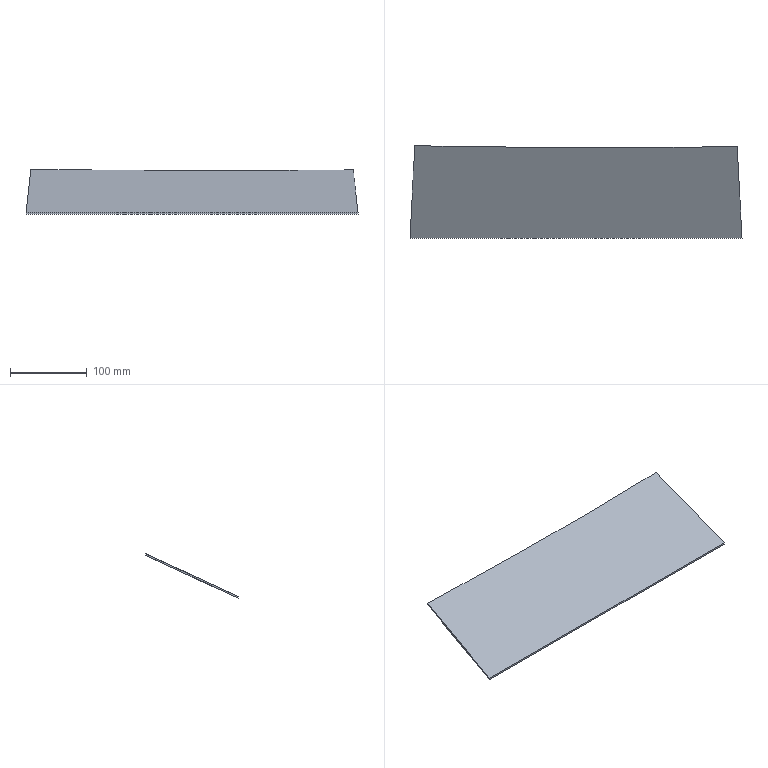Part | NX | features solid 2 | 1 solid | 6 faces | box 431.972 x 120.175 x 58.245 mm | volume 111226 mm3 | plane 5 | spline 1
STEP:
#1=CARTESIAN_POINT('',(-249.743,-364.825,19.75));
#2=VERTEX_POINT('',#1);
#3=CARTESIAN_POINT('',(169.68,-365.715,19.335));
#4=VERTEX_POINT('',#3);
#5=CARTESIAN_POINT('',(-249.743,-364.825,19.75));
#6=CARTESIAN_POINT('',(-232.267,-365.051,19.645));
#7=CARTESIAN_POINT('',(-206.054,-365.258,19.548));
#8=CARTESIAN_POINT('',(-171.103,-365.659,19.361));
#9=CARTESIAN_POINT('',(-136.154,-366.255,19.083));
#10=CARTESIAN_POINT('',(-101.203,-366.757,18.849));
#11=CARTESIAN_POINT('',(-66.253,-367.313,18.59));
#12=CARTESIAN_POINT('',(-40.041,-367.708,18.406));
#13=CARTESIAN_POINT('',(-13.826,-367.635,18.44));
#14=CARTESIAN_POINT('',(12.388,-367.617,18.448));
#15=CARTESIAN_POINT('',(38.602,-367.689,18.414));
#16=CARTESIAN_POINT('',(64.817,-367.364,18.566));
#17=CARTESIAN_POINT('',(91.033,-366.909,18.778));
#18=CARTESIAN_POINT('',(117.249,-366.489,18.974));
#19=CARTESIAN_POINT('',(143.464,-366.132,19.141));
#20=CARTESIAN_POINT('',(160.941,-365.843,19.275));
#21=CARTESIAN_POINT('',(169.68,-365.715,19.335));
#22=B_SPLINE_CURVE_WITH_KNOTS('',3,(#5,#6,#7,#8,#9,#10,#11,#12,#13,#14,#15,#16,#17,#18,#19,#20,#21),.UNSPECIFIED.,.F.,.F.,(4,1,1,1,1,1,1,1,1,1,1,1,1,1,4),(0.5223,0.5724,0.5974,0.6224,0.6725,0.6975,0.7226,0.7476,0.7726,0.7977,0.8227,0.8477,0.8727,0.8978,0.9228),.UNSPECIFIED.);
#23=EDGE_CURVE('',#2,#4,#22,.T.);
#24=ORIENTED_EDGE('',*,*,#23,.T.);
#25=CARTESIAN_POINT('',(169.68,-365.715,17.128));
#26=VERTEX_POINT('',#25);
#27=CARTESIAN_POINT('',(169.68,-365.715,18.403));
#28=DIRECTION('',(0.,0.,-1.));
#29=VECTOR('',#28,1000.);
#30=LINE('',#27,#29);
#31=EDGE_CURVE('',#4,#26,#30,.T.);
#32=ORIENTED_EDGE('',*,*,#31,.T.);
#33=CARTESIAN_POINT('',(-249.743,-364.825,17.543));
#34=VERTEX_POINT('',#33);
#35=CARTESIAN_POINT('',(-249.743,-364.825,17.543));
#36=CARTESIAN_POINT('',(-232.263,-365.051,17.438));
#37=CARTESIAN_POINT('',(-206.047,-365.258,17.342));
#38=CARTESIAN_POINT('',(-171.09,-365.659,17.154));
#39=CARTESIAN_POINT('',(-136.129,-366.256,16.876));
#40=CARTESIAN_POINT('',(-101.17,-366.757,16.642));
#41=CARTESIAN_POINT('',(-66.209,-367.314,16.383));
#42=CARTESIAN_POINT('',(-39.99,-367.709,16.199));
#43=CARTESIAN_POINT('',(-13.778,-367.634,16.233));
#44=CARTESIAN_POINT('',(12.435,-367.617,16.241));
#45=CARTESIAN_POINT('',(38.649,-367.689,16.208));
#46=CARTESIAN_POINT('',(64.856,-367.364,16.36));
#47=CARTESIAN_POINT('',(91.061,-366.909,16.572));
#48=CARTESIAN_POINT('',(117.267,-366.489,16.767));
#49=CARTESIAN_POINT('',(143.474,-366.131,16.934));
#50=CARTESIAN_POINT('',(160.944,-365.843,17.069));
#51=CARTESIAN_POINT('',(169.68,-365.715,17.128));
#52=B_SPLINE_CURVE_WITH_KNOTS('',3,(#35,#36,#37,#38,#39,#40,#41,#42,#43,#44,#45,#46,#47,#48,#49,#50,#51),.UNSPECIFIED.,.F.,.F.,(4,1,1,1,1,1,1,1,1,1,1,1,1,1,4),(0.5017,0.5492,0.573,0.5967,0.6442,0.6679,0.6917,0.7154,0.7392,0.7629,0.7867,0.8104,0.8342,0.8579,0.8816),.UNSPECIFIED.);
#53=EDGE_CURVE('',#34,#26,#52,.T.);
#54=ORIENTED_EDGE('',*,*,#53,.F.);
#55=CARTESIAN_POINT('',(-249.743,-364.825,32.28));
#56=DIRECTION('',(0.,0.,-1.));
#57=VECTOR('',#56,1000.);
#58=LINE('',#55,#57);
#59=EDGE_CURVE('',#34,#2,#58,.F.);
#60=ORIENTED_EDGE('',*,*,#59,.T.);
#61=EDGE_LOOP('',(#24,#32,#54,#60));
#62=FACE_BOUND('',#61,.T.);
#63=CARTESIAN_POINT('',(169.68,-365.715,19.773));
#64=CARTESIAN_POINT('',(169.68,-365.715,15.99));
#65=CARTESIAN_POINT('',(160.942,-365.843,19.773));
#66=CARTESIAN_POINT('',(160.942,-365.843,15.99));
#67=CARTESIAN_POINT('',(143.467,-366.132,19.773));
#68=CARTESIAN_POINT('',(143.467,-366.132,15.99));
#69=CARTESIAN_POINT('',(117.253,-366.489,19.773));
#70=CARTESIAN_POINT('',(117.253,-366.489,15.99));
#71=CARTESIAN_POINT('',(91.041,-366.909,19.773));
#72=CARTESIAN_POINT('',(91.041,-366.909,15.99));
#73=CARTESIAN_POINT('',(64.829,-367.364,19.773));
#74=CARTESIAN_POINT('',(64.829,-367.364,15.99));
#75=CARTESIAN_POINT('',(38.614,-367.689,19.773));
#76=CARTESIAN_POINT('',(38.614,-367.689,15.99));
#77=CARTESIAN_POINT('',(12.398,-367.617,19.773));
#78=CARTESIAN_POINT('',(12.398,-367.617,15.99));
#79=CARTESIAN_POINT('',(-13.818,-367.635,19.773));
#80=CARTESIAN_POINT('',(-13.818,-367.635,15.99));
#81=CARTESIAN_POINT('',(-40.034,-367.708,19.773));
#82=CARTESIAN_POINT('',(-40.034,-367.708,15.99));
#83=CARTESIAN_POINT('',(-66.248,-367.313,19.773));
#84=CARTESIAN_POINT('',(-66.248,-367.313,15.99));
#85=CARTESIAN_POINT('',(-101.199,-366.757,19.773));
#86=CARTESIAN_POINT('',(-101.199,-366.757,15.99));
#87=CARTESIAN_POINT('',(-136.149,-366.255,19.773));
#88=CARTESIAN_POINT('',(-136.149,-366.255,15.99));
#89=CARTESIAN_POINT('',(-171.099,-365.659,19.773));
#90=CARTESIAN_POINT('',(-171.099,-365.659,15.99));
#91=CARTESIAN_POINT('',(-206.051,-365.258,19.773));
#92=CARTESIAN_POINT('',(-206.051,-365.258,15.99));
#93=CARTESIAN_POINT('',(-232.267,-365.051,19.773));
#94=CARTESIAN_POINT('',(-232.267,-365.051,15.99));
#95=CARTESIAN_POINT('',(-249.743,-364.825,19.773));
#96=CARTESIAN_POINT('',(-249.743,-364.825,15.99));
#97=B_SPLINE_SURFACE_WITH_KNOTS('',3,1,((#63,#64),(#65,#66),(#67,#68),(#69,#70),(#71,#72),(#73,#74),(#75,#76),(#77,#78),(#79,#80),(#81,#82),(#83,#84),(#85,#86),(#87,#88),(#89,#90),(#91,#92),(#93,#94),(#95,#96)),.SURF_OF_LINEAR_EXTRUSION.,.F.,.F.,.F.,(4,1,1,1,1,1,1,1,1,1,1,1,1,1,4),(2,2),(0.1805,0.1862,0.192,0.1978,0.2035,0.2093,0.2151,0.2208,0.2266,0.2324,0.2381,0.2497,0.2554,0.2612,0.2727),(0.,1.),.UNSPECIFIED.);
#98=ADVANCED_FACE('',(#62),#97,.F.);
#99=ORIENTED_EDGE('',*,*,#53,.T.);
#100=CARTESIAN_POINT('',(175.931,-485.,-38.495));
#101=VERTEX_POINT('',#100);
#102=CARTESIAN_POINT('',(195.802,-864.162,-215.301));
#103=DIRECTION('',(0.04744,-0.9053,-0.4221));
#104=VECTOR('',#103,1000.);
#105=LINE('',#102,#104);
#106=EDGE_CURVE('',#26,#101,#105,.T.);
#107=ORIENTED_EDGE('',*,*,#106,.T.);
#108=CARTESIAN_POINT('',(-256.041,-485.,-38.495));
#109=VERTEX_POINT('',#108);
#110=CARTESIAN_POINT('',(-705.,-485.,-38.495));
#111=DIRECTION('',(-1.,0.,0.));
#112=VECTOR('',#111,1000.);
#113=LINE('',#110,#112);
#114=EDGE_CURVE('',#109,#101,#113,.F.);
#115=ORIENTED_EDGE('',*,*,#114,.F.);
#116=CARTESIAN_POINT('',(-278.906,-921.282,-241.937));
#117=DIRECTION('',(0.04745,0.9053,0.4221));
#118=VECTOR('',#117,1000.);
#119=LINE('',#116,#118);
#120=EDGE_CURVE('',#109,#34,#119,.T.);
#121=ORIENTED_EDGE('',*,*,#120,.T.);
#122=EDGE_LOOP('',(#99,#107,#115,#121));
#123=FACE_BOUND('',#122,.T.);
#124=CARTESIAN_POINT('',(-705.,-902.939,-233.384));
#125=DIRECTION('',(0.,-0.4226,0.9063));
#126=DIRECTION('',(1.,0.,0.));
#127=AXIS2_PLACEMENT_3D('',#124,#125,#126);
#128=PLANE('',#127);
#129=ADVANCED_FACE('',(#123),#128,.F.);
#130=CARTESIAN_POINT('',(175.931,-485.,-36.288));
#131=VERTEX_POINT('',#130);
#132=CARTESIAN_POINT('',(195.846,-865.006,-213.488));
#133=DIRECTION('',(0.04744,-0.9053,-0.4221));
#134=VECTOR('',#133,1000.);
#135=LINE('',#132,#134);
#136=EDGE_CURVE('',#4,#131,#135,.T.);
#137=ORIENTED_EDGE('',*,*,#136,.F.);
#138=ORIENTED_EDGE('',*,*,#23,.F.);
#139=CARTESIAN_POINT('',(-256.041,-485.,-36.288));
#140=VERTEX_POINT('',#139);
#141=CARTESIAN_POINT('',(-278.951,-922.126,-240.124));
#142=DIRECTION('',(0.04745,0.9053,0.4221));
#143=VECTOR('',#142,1000.);
#144=LINE('',#141,#143);
#145=EDGE_CURVE('',#140,#2,#144,.T.);
#146=ORIENTED_EDGE('',*,*,#145,.F.);
#147=CARTESIAN_POINT('',(-705.,-485.,-36.288));
#148=DIRECTION('',(-1.,0.,0.));
#149=VECTOR('',#148,1000.);
#150=LINE('',#147,#149);
#151=EDGE_CURVE('',#140,#131,#150,.F.);
#152=ORIENTED_EDGE('',*,*,#151,.T.);
#153=EDGE_LOOP('',(#137,#138,#146,#152));
#154=FACE_BOUND('',#153,.T.);
#155=CARTESIAN_POINT('',(-705.,-903.785,-231.571));
#156=DIRECTION('',(0.,-0.4226,0.9063));
#157=DIRECTION('',(1.,0.,0.));
#158=AXIS2_PLACEMENT_3D('',#155,#156,#157);
#159=PLANE('',#158);
#160=ADVANCED_FACE('',(#154),#159,.T.);
#161=CARTESIAN_POINT('',(175.931,-485.,-55.));
#162=DIRECTION('',(0.,0.,1.));
#163=VECTOR('',#162,1000.);
#164=LINE('',#161,#163);
#165=EDGE_CURVE('',#131,#101,#164,.F.);
#166=ORIENTED_EDGE('',*,*,#165,.F.);
#167=ORIENTED_EDGE('',*,*,#151,.F.);
#168=CARTESIAN_POINT('',(-256.041,-485.,-55.));
#169=DIRECTION('',(0.,0.,-1.));
#170=VECTOR('',#169,1000.);
#171=LINE('',#168,#170);
#172=EDGE_CURVE('',#109,#140,#171,.F.);
#173=ORIENTED_EDGE('',*,*,#172,.F.);
#174=ORIENTED_EDGE('',*,*,#114,.T.);
#175=EDGE_LOOP('',(#166,#167,#173,#174));
#176=FACE_BOUND('',#175,.T.);
#177=CARTESIAN_POINT('',(691.22,-485.,-55.));
#178=DIRECTION('',(0.,1.,0.));
#179=DIRECTION('',(-1.,0.,0.));
#180=AXIS2_PLACEMENT_3D('',#177,#178,#179);
#181=PLANE('',#180);
#182=ADVANCED_FACE('',(#176),#181,.F.);
#183=ORIENTED_EDGE('',*,*,#172,.T.);
#184=ORIENTED_EDGE('',*,*,#145,.T.);
#185=ORIENTED_EDGE('',*,*,#59,.F.);
#186=ORIENTED_EDGE('',*,*,#120,.F.);
#187=EDGE_LOOP('',(#183,#184,#185,#186));
#188=FACE_BOUND('',#187,.T.);
#189=CARTESIAN_POINT('',(-254.993,-465.,-65.));
#190=DIRECTION('',(0.9986,-0.05234,0.));
#191=DIRECTION('',(0.05234,0.9986,0.));
#192=AXIS2_PLACEMENT_3D('',#189,#190,#191);
#193=PLANE('',#192);
#194=ADVANCED_FACE('',(#188),#193,.F.);
#195=ORIENTED_EDGE('',*,*,#136,.T.);
#196=ORIENTED_EDGE('',*,*,#165,.T.);
#197=ORIENTED_EDGE('',*,*,#106,.F.);
#198=ORIENTED_EDGE('',*,*,#31,.F.);
#199=EDGE_LOOP('',(#195,#196,#197,#198));
#200=FACE_BOUND('',#199,.T.);
#201=CARTESIAN_POINT('',(175.075,-468.664,-65.));
#202=DIRECTION('',(-0.9986,-0.05234,0.));
#203=DIRECTION('',(0.05234,-0.9986,0.));
#204=AXIS2_PLACEMENT_3D('',#201,#202,#203);
#205=PLANE('',#204);
#206=ADVANCED_FACE('',(#200),#205,.F.);
#207=CLOSED_SHELL('',(#98,#129,#160,#182,#194,#206));
#208=MANIFOLD_SOLID_BREP('',#207);
#209=(LENGTH_UNIT()NAMED_UNIT(*)SI_UNIT(.MILLI.,.METRE.));
#210=UNCERTAINTY_MEASURE_WITH_UNIT(LENGTH_MEASURE(0.0508),#209,'','');
#211=(NAMED_UNIT(*)PLANE_ANGLE_UNIT()SI_UNIT($,.RADIAN.));
#212=(NAMED_UNIT(*)SI_UNIT($,.STERADIAN.)SOLID_ANGLE_UNIT());
#213=(GEOMETRIC_REPRESENTATION_CONTEXT(3)GLOBAL_UNCERTAINTY_ASSIGNED_CONTEXT((#210))GLOBAL_UNIT_ASSIGNED_CONTEXT((#209,#211,#212))REPRESENTATION_CONTEXT('',''));
#214=ADVANCED_BREP_SHAPE_REPRESENTATION('',(#208),#213);